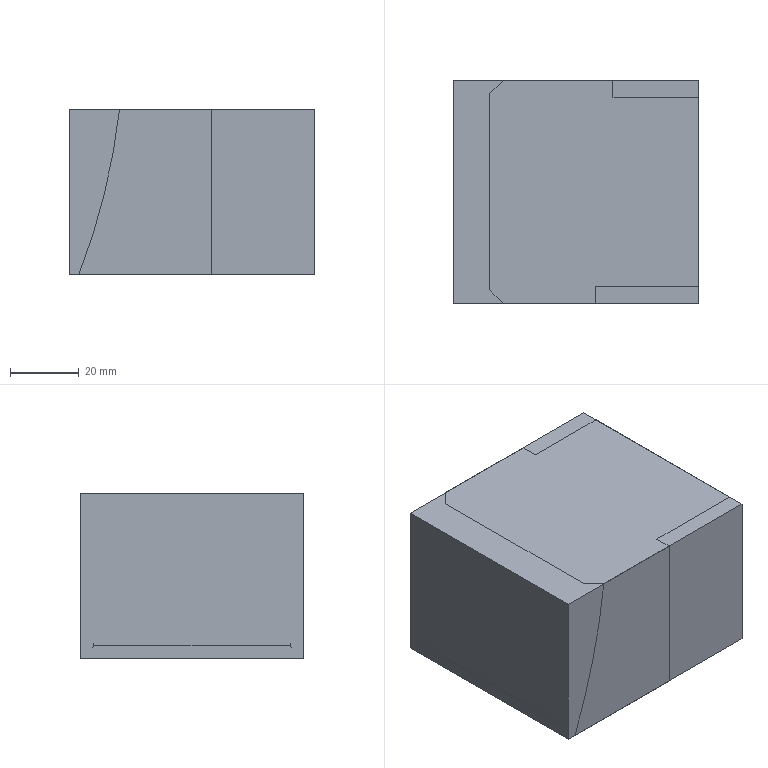NC program | NX | posted with a generic post | part box 71.51 x 65 x 48 mm
Lines 21 to 852 of 3379:
(ZLEVEL_PROFILE_COPY , TOOL : D10)
N40 T10 M6
N42 G54
N44 G17 G0 G90 X-28.587 Y-37.6 B0. C0. S9500 M3
N46 G43 Z30. H10
N48 Z1.5
N50 G94 G1 X-36.309 Z1.095 F2000.
N52 X-37.653 Y-37.266 Z1.023
N54 X-38.859 Y-36.584 Z0.95
N56 X-39.839 Y-35.604 Z0.877
N58 X-40.521 Y-34.398 Z0.805
N60 X-40.855 Y-33.054 Z0.732
N62 Y-32.5 Z0.703
N64 Y0. Z-1.
N66 Y32.5
N68 G2 X-35.755 Y37.6 R5.1
N70 G1 X35.755
N72 G2 X40.855 Y32.5 R5.1
N74 G1 Y-32.5
N76 G2 X35.755 Y-37.6 R5.1
N78 G1 X-35.755
N80 G2 X-40.855 Y-32.5 R5.1
N82 G1 Y0.
N84 Y32.5 Z-1.107
N86 X-40.83 Y33. Z-1.108
N88 X-40.757 Y33.495 Z-1.11
N90 X-40.635 Y33.98 Z-1.111
N92 X-40.467 Y34.452 Z-1.113
N94 X-40.253 Y34.904 Z-1.115
N96 X-39.996 Y35.333 Z-1.116
N98 X-39.697 Y35.735 Z-1.118
N100 X-39.361 Y36.106 Z-1.12
N102 X-38.99 Y36.442 Z-1.121
N104 X-38.588 Y36.74 Z-1.123
N106 X-38.159 Y36.998 Z-1.125
N108 X-37.707 Y37.212 Z-1.126
N110 X-37.235 Y37.38 Z-1.128
N112 X-36.75 Y37.502 Z-1.129
N114 X-36.255 Y37.575 Z-1.131
N116 X-35.755 Y37.6 Z-1.133
N118 X35.755 Z-1.367
N120 X36.255 Y37.575 Z-1.369
N122 X36.75 Y37.502 Z-1.371
N124 X37.235 Y37.38 Z-1.372
N126 X37.707 Y37.212 Z-1.374
N128 X38.159 Y36.998 Z-1.375
N130 X38.588 Y36.74 Z-1.377
N132 X38.99 Y36.442 Z-1.379
N134 X39.361 Y36.106 Z-1.38
N136 X39.697 Y35.735 Z-1.382
N138 X39.996 Y35.333 Z-1.384
N140 X40.253 Y34.904 Z-1.385
N142 X40.467 Y34.452 Z-1.387
N144 X40.635 Y33.98 Z-1.389
N146 X40.757 Y33.495 Z-1.39
N148 X40.83 Y33. Z-1.392
N150 X40.855 Y32.5 Z-1.393
N152 Y-32.5 Z-1.607
N154 X40.83 Y-33. Z-1.608
N156 X40.757 Y-33.495 Z-1.61
N158 X40.635 Y-33.98 Z-1.611
N160 X40.467 Y-34.452 Z-1.613
N162 X40.253 Y-34.904 Z-1.615
N164 X39.996 Y-35.333 Z-1.616
N166 X39.697 Y-35.735 Z-1.618
N168 X39.361 Y-36.106 Z-1.62
N170 X38.99 Y-36.442 Z-1.621
N172 X38.588 Y-36.74 Z-1.623
N174 X38.159 Y-36.998 Z-1.625
N176 X37.707 Y-37.212 Z-1.626
N178 X37.235 Y-37.38 Z-1.628
N180 X36.75 Y-37.502 Z-1.629
N182 X36.255 Y-37.575 Z-1.631
N184 X35.755 Y-37.6 Z-1.633
N186 X-35.755 Z-1.867
N188 X-36.255 Y-37.575 Z-1.869
N190 X-36.75 Y-37.502 Z-1.871
N192 X-37.235 Y-37.38 Z-1.872
N194 X-37.707 Y-37.212 Z-1.874
N196 X-38.159 Y-36.998 Z-1.875
N198 X-38.588 Y-36.74 Z-1.877
N200 X-38.99 Y-36.442 Z-1.879
N202 X-39.361 Y-36.106 Z-1.88
N204 X-39.697 Y-35.735 Z-1.882
N206 X-39.996 Y-35.333 Z-1.884
N208 X-40.253 Y-34.904 Z-1.885
N210 X-40.467 Y-34.452 Z-1.887
N212 X-40.635 Y-33.98 Z-1.889
N214 X-40.757 Y-33.495 Z-1.89
N216 X-40.83 Y-33. Z-1.892
N218 X-40.855 Y-32.5 Z-1.893
N220 Y0. Z-2.
N222 Y32.5 Z-2.107
N224 X-40.83 Y33. Z-2.108
N226 X-40.757 Y33.495 Z-2.11
N228 X-40.635 Y33.98 Z-2.111
N230 X-40.467 Y34.452 Z-2.113
N232 X-40.253 Y34.904 Z-2.115
N234 X-39.996 Y35.333 Z-2.116
N236 X-39.697 Y35.735 Z-2.118
N238 X-39.361 Y36.106 Z-2.12
N240 X-38.99 Y36.442 Z-2.121
N242 X-38.588 Y36.74 Z-2.123
N244 X-38.159 Y36.998 Z-2.125
N246 X-37.707 Y37.212 Z-2.126
N248 X-37.235 Y37.38 Z-2.128
N250 X-36.75 Y37.502 Z-2.129
N252 X-36.255 Y37.575 Z-2.131
N254 X-35.755 Y37.6 Z-2.133
N256 X35.755 Z-2.367
N258 X36.255 Y37.575 Z-2.369
N260 X36.75 Y37.502 Z-2.371
N262 X37.235 Y37.38 Z-2.372
N264 X37.707 Y37.212 Z-2.374
N266 X38.159 Y36.998 Z-2.375
N268 X38.588 Y36.74 Z-2.377
N270 X38.99 Y36.442 Z-2.379
N272 X39.361 Y36.106 Z-2.38
N274 X39.697 Y35.735 Z-2.382
N276 X39.996 Y35.333 Z-2.384
N278 X40.253 Y34.904 Z-2.385
N280 X40.467 Y34.452 Z-2.387
N282 X40.635 Y33.98 Z-2.389
N284 X40.757 Y33.495 Z-2.39
N286 X40.83 Y33. Z-2.392
N288 X40.855 Y32.5 Z-2.393
N290 Y-32.5 Z-2.607
N292 X40.83 Y-33. Z-2.608
N294 X40.757 Y-33.495 Z-2.61
N296 X40.635 Y-33.98 Z-2.611
N298 X40.467 Y-34.452 Z-2.613
N300 X40.253 Y-34.904 Z-2.615
N302 X39.996 Y-35.333 Z-2.616
N304 X39.697 Y-35.735 Z-2.618
N306 X39.361 Y-36.106 Z-2.62
N308 X38.99 Y-36.442 Z-2.621
N310 X38.588 Y-36.74 Z-2.623
N312 X38.159 Y-36.998 Z-2.625
N314 X37.707 Y-37.212 Z-2.626
N316 X37.235 Y-37.38 Z-2.628
N318 X36.75 Y-37.502 Z-2.629
N320 X36.255 Y-37.575 Z-2.631
N322 X35.755 Y-37.6 Z-2.633
N324 X-35.755 Z-2.867
N326 X-36.255 Y-37.575 Z-2.869
N328 X-36.75 Y-37.502 Z-2.871
N330 X-37.235 Y-37.38 Z-2.872
N332 X-37.707 Y-37.212 Z-2.874
N334 X-38.159 Y-36.998 Z-2.875
N336 X-38.588 Y-36.74 Z-2.877
N338 X-38.99 Y-36.442 Z-2.879
N340 X-39.361 Y-36.106 Z-2.88
N342 X-39.697 Y-35.735 Z-2.882
N344 X-39.996 Y-35.333 Z-2.884
N346 X-40.253 Y-34.904 Z-2.885
N348 X-40.467 Y-34.452 Z-2.887
N350 X-40.635 Y-33.98 Z-2.889
N352 X-40.757 Y-33.495 Z-2.89
N354 X-40.83 Y-33. Z-2.892
N356 X-40.855 Y-32.5 Z-2.893
N358 Y0. Z-3.
N360 Y32.5 Z-3.107
N362 X-40.83 Y33. Z-3.108
N364 X-40.757 Y33.495 Z-3.11
N366 X-40.635 Y33.98 Z-3.111
N368 X-40.467 Y34.452 Z-3.113
N370 X-40.253 Y34.904 Z-3.115
N372 X-39.996 Y35.333 Z-3.116
N374 X-39.697 Y35.735 Z-3.118
N376 X-39.361 Y36.106 Z-3.12
N378 X-38.99 Y36.442 Z-3.121
N380 X-38.588 Y36.74 Z-3.123
N382 X-38.159 Y36.998 Z-3.125
N384 X-37.707 Y37.212 Z-3.126
N386 X-37.235 Y37.38 Z-3.128
N388 X-36.75 Y37.502 Z-3.129
N390 X-36.255 Y37.575 Z-3.131
N392 X-35.755 Y37.6 Z-3.133
N394 X35.755 Z-3.367
N396 X36.255 Y37.575 Z-3.369
N398 X36.75 Y37.502 Z-3.371
N400 X37.235 Y37.38 Z-3.372
N402 X37.707 Y37.212 Z-3.374
N404 X38.159 Y36.998 Z-3.375
N406 X38.588 Y36.74 Z-3.377
N408 X38.99 Y36.442 Z-3.379
N410 X39.361 Y36.106 Z-3.38
N412 X39.697 Y35.735 Z-3.382
N414 X39.996 Y35.333 Z-3.384
N416 X40.253 Y34.904 Z-3.385
N418 X40.467 Y34.452 Z-3.387
N420 X40.635 Y33.98 Z-3.389
N422 X40.757 Y33.495 Z-3.39
N424 X40.83 Y33. Z-3.392
N426 X40.855 Y32.5 Z-3.393
N428 Y-32.5 Z-3.607
N430 X40.83 Y-33. Z-3.608
N432 X40.757 Y-33.495 Z-3.61
N434 X40.635 Y-33.98 Z-3.611
N436 X40.467 Y-34.452 Z-3.613
N438 X40.253 Y-34.904 Z-3.615
N440 X39.996 Y-35.333 Z-3.616
N442 X39.697 Y-35.735 Z-3.618
N444 X39.361 Y-36.106 Z-3.62
N446 X38.99 Y-36.442 Z-3.621
N448 X38.588 Y-36.74 Z-3.623
N450 X38.159 Y-36.998 Z-3.625
N452 X37.707 Y-37.212 Z-3.626
N454 X37.235 Y-37.38 Z-3.628
N456 X36.75 Y-37.502 Z-3.629
N458 X36.255 Y-37.575 Z-3.631
N460 X35.755 Y-37.6 Z-3.633
N462 X-35.755 Z-3.867
N464 X-36.255 Y-37.575 Z-3.869
N466 X-36.75 Y-37.502 Z-3.871
N468 X-37.235 Y-37.38 Z-3.872
N470 X-37.707 Y-37.212 Z-3.874
N472 X-38.159 Y-36.998 Z-3.875
N474 X-38.588 Y-36.74 Z-3.877
N476 X-38.99 Y-36.442 Z-3.879
N478 X-39.361 Y-36.106 Z-3.88
N480 X-39.697 Y-35.735 Z-3.882
N482 X-39.996 Y-35.333 Z-3.884
N484 X-40.253 Y-34.904 Z-3.885
N486 X-40.467 Y-34.452 Z-3.887
N488 X-40.635 Y-33.98 Z-3.889
N490 X-40.757 Y-33.495 Z-3.89
N492 X-40.83 Y-33. Z-3.892
N494 X-40.855 Y-32.5 Z-3.893
N496 Y0. Z-4.
N498 Y32.5 Z-4.107
N500 X-40.83 Y33. Z-4.108
N502 X-40.757 Y33.495 Z-4.11
N504 X-40.635 Y33.98 Z-4.111
N506 X-40.467 Y34.452 Z-4.113
N508 X-40.253 Y34.904 Z-4.115
N510 X-39.996 Y35.333 Z-4.116
N512 X-39.697 Y35.735 Z-4.118
N514 X-39.361 Y36.106 Z-4.12
N516 X-38.99 Y36.442 Z-4.121
N518 X-38.588 Y36.74 Z-4.123
N520 X-38.159 Y36.998 Z-4.125
N522 X-37.707 Y37.212 Z-4.126
N524 X-37.235 Y37.38 Z-4.128
N526 X-36.75 Y37.502 Z-4.129
N528 X-36.255 Y37.575 Z-4.131
N530 X-35.755 Y37.6 Z-4.133
N532 X35.755 Z-4.367
N534 X36.255 Y37.575 Z-4.369
N536 X36.75 Y37.502 Z-4.371
N538 X37.235 Y37.38 Z-4.372
N540 X37.707 Y37.212 Z-4.374
N542 X38.159 Y36.998 Z-4.375
N544 X38.588 Y36.74 Z-4.377
N546 X38.99 Y36.442 Z-4.379
N548 X39.361 Y36.106 Z-4.38
N550 X39.697 Y35.735 Z-4.382
N552 X39.996 Y35.333 Z-4.384
N554 X40.253 Y34.904 Z-4.385
N556 X40.467 Y34.452 Z-4.387
N558 X40.635 Y33.98 Z-4.389
N560 X40.757 Y33.495 Z-4.39
N562 X40.83 Y33. Z-4.392
N564 X40.855 Y32.5 Z-4.393
N566 Y-32.5 Z-4.607
N568 X40.83 Y-33. Z-4.608
N570 X40.757 Y-33.495 Z-4.61
N572 X40.635 Y-33.98 Z-4.611
N574 X40.467 Y-34.452 Z-4.613
N576 X40.253 Y-34.904 Z-4.615
N578 X39.996 Y-35.333 Z-4.616
N580 X39.697 Y-35.735 Z-4.618
N582 X39.361 Y-36.106 Z-4.62
N584 X38.99 Y-36.442 Z-4.621
N586 X38.588 Y-36.74 Z-4.623
N588 X38.159 Y-36.998 Z-4.625
N590 X37.707 Y-37.212 Z-4.626
N592 X37.235 Y-37.38 Z-4.628
N594 X36.75 Y-37.502 Z-4.629
N596 X36.255 Y-37.575 Z-4.631
N598 X35.755 Y-37.6 Z-4.633
N600 X-35.755 Z-4.867
N602 X-36.255 Y-37.575 Z-4.869
N604 X-36.75 Y-37.502 Z-4.871
N606 X-37.235 Y-37.38 Z-4.872
N608 X-37.707 Y-37.212 Z-4.874
N610 X-38.159 Y-36.998 Z-4.875
N612 X-38.588 Y-36.74 Z-4.877
N614 X-38.99 Y-36.442 Z-4.879
N616 X-39.361 Y-36.106 Z-4.88
N618 X-39.697 Y-35.735 Z-4.882
N620 X-39.996 Y-35.333 Z-4.884
N622 X-40.253 Y-34.904 Z-4.885
N624 X-40.467 Y-34.452 Z-4.887
N626 X-40.635 Y-33.98 Z-4.889
N628 X-40.757 Y-33.495 Z-4.89
N630 X-40.83 Y-33. Z-4.892
N632 X-40.855 Y-32.5 Z-4.893
N634 Y0. Z-5.
N636 Y32.5 Z-5.107
N638 X-40.83 Y33. Z-5.108
N640 X-40.757 Y33.495 Z-5.11
N642 X-40.635 Y33.98 Z-5.111
N644 X-40.467 Y34.452 Z-5.113
N646 X-40.253 Y34.904 Z-5.115
N648 X-39.996 Y35.333 Z-5.116
N650 X-39.697 Y35.735 Z-5.118
N652 X-39.361 Y36.106 Z-5.12
N654 X-38.99 Y36.442 Z-5.121
N656 X-38.588 Y36.74 Z-5.123
N658 X-38.159 Y36.998 Z-5.125
N660 X-37.707 Y37.212 Z-5.126
N662 X-37.235 Y37.38 Z-5.128
N664 X-36.75 Y37.502 Z-5.129
N666 X-36.255 Y37.575 Z-5.131
N668 X-35.755 Y37.6 Z-5.133
N670 X35.755 Z-5.367
N672 X36.255 Y37.575 Z-5.369
N674 X36.75 Y37.502 Z-5.371
N676 X37.235 Y37.38 Z-5.372
N678 X37.707 Y37.212 Z-5.374
N680 X38.159 Y36.998 Z-5.375
N682 X38.588 Y36.74 Z-5.377
N684 X38.99 Y36.442 Z-5.379
N686 X39.361 Y36.106 Z-5.38
N688 X39.697 Y35.735 Z-5.382
N690 X39.996 Y35.333 Z-5.384
N692 X40.253 Y34.904 Z-5.385
N694 X40.467 Y34.452 Z-5.387
N696 X40.635 Y33.98 Z-5.389
N698 X40.757 Y33.495 Z-5.39
N700 X40.83 Y33. Z-5.392
N702 X40.855 Y32.5 Z-5.393
N704 Y-32.5 Z-5.607
N706 X40.83 Y-33. Z-5.608
N708 X40.757 Y-33.495 Z-5.61
N710 X40.635 Y-33.98 Z-5.611
N712 X40.467 Y-34.452 Z-5.613
N714 X40.253 Y-34.904 Z-5.615
N716 X39.996 Y-35.333 Z-5.616
N718 X39.697 Y-35.735 Z-5.618
N720 X39.361 Y-36.106 Z-5.62
N722 X38.99 Y-36.442 Z-5.621
N724 X38.588 Y-36.74 Z-5.623
N726 X38.159 Y-36.998 Z-5.625
N728 X37.707 Y-37.212 Z-5.626
N730 X37.235 Y-37.38 Z-5.628
N732 X36.75 Y-37.502 Z-5.629
N734 X36.255 Y-37.575 Z-5.631
N736 X35.755 Y-37.6 Z-5.633
N738 X-35.755 Z-5.867
N740 X-36.255 Y-37.575 Z-5.869
N742 X-36.75 Y-37.502 Z-5.871
N744 X-37.235 Y-37.38 Z-5.872
N746 X-37.707 Y-37.212 Z-5.874
N748 X-38.159 Y-36.998 Z-5.875
N750 X-38.588 Y-36.74 Z-5.877
N752 X-38.99 Y-36.442 Z-5.879
N754 X-39.361 Y-36.106 Z-5.88
N756 X-39.697 Y-35.735 Z-5.882
N758 X-39.996 Y-35.333 Z-5.884
N760 X-40.253 Y-34.904 Z-5.885
N762 X-40.467 Y-34.452 Z-5.887
N764 X-40.635 Y-33.98 Z-5.889
N766 X-40.757 Y-33.495 Z-5.89
N768 X-40.83 Y-33. Z-5.892
N770 X-40.855 Y-32.5 Z-5.893
N772 Y0. Z-6.
N774 Y32.5 Z-6.107
N776 X-40.83 Y33. Z-6.108
N778 X-40.757 Y33.495 Z-6.11
N780 X-40.635 Y33.98 Z-6.111
N782 X-40.467 Y34.452 Z-6.113
N784 X-40.253 Y34.904 Z-6.115
N786 X-39.996 Y35.333 Z-6.116
N788 X-39.697 Y35.735 Z-6.118
N790 X-39.361 Y36.106 Z-6.12
N792 X-38.99 Y36.442 Z-6.121
N794 X-38.588 Y36.74 Z-6.123
N796 X-38.159 Y36.998 Z-6.125
N798 X-37.707 Y37.212 Z-6.126
N800 X-37.235 Y37.38 Z-6.128
N802 X-36.75 Y37.502 Z-6.129
N804 X-36.255 Y37.575 Z-6.131
N806 X-35.755 Y37.6 Z-6.133
N808 X35.755 Z-6.367
N810 X36.255 Y37.575 Z-6.369
N812 X36.75 Y37.502 Z-6.371
N814 X37.235 Y37.38 Z-6.372
N816 X37.707 Y37.212 Z-6.374
N818 X38.159 Y36.998 Z-6.375
N820 X38.588 Y36.74 Z-6.377
N822 X38.99 Y36.442 Z-6.379
N824 X39.361 Y36.106 Z-6.38
N826 X39.697 Y35.735 Z-6.382
N828 X39.996 Y35.333 Z-6.384
N830 X40.253 Y34.904 Z-6.385
N832 X40.467 Y34.452 Z-6.387
N834 X40.635 Y33.98 Z-6.389
N836 X40.757 Y33.495 Z-6.39
N838 X40.83 Y33. Z-6.392
N840 X40.855 Y32.5 Z-6.393
N842 Y-32.5 Z-6.607
N844 X40.83 Y-33. Z-6.608
N846 X40.757 Y-33.495 Z-6.61
N848 X40.635 Y-33.98 Z-6.611
N850 X40.467 Y-34.452 Z-6.613
N852 X40.253 Y-34.904 Z-6.615
N854 X39.996 Y-35.333 Z-6.616
N856 X39.697 Y-35.735 Z-6.618
N858 X39.361 Y-36.106 Z-6.62
N860 X38.99 Y-36.442 Z-6.621
N862 X38.588 Y-36.74 Z-6.623
N864 X38.159 Y-36.998 Z-6.625
N866 X37.707 Y-37.212 Z-6.626
N868 X37.235 Y-37.38 Z-6.628
N870 X36.75 Y-37.502 Z-6.629
N872 X36.255 Y-37.575 Z-6.631
N874 X35.755 Y-37.6 Z-6.633
N876 X-35.755 Z-6.867
N878 X-36.255 Y-37.575 Z-6.869
N880 X-36.75 Y-37.502 Z-6.871
N882 X-37.235 Y-37.38 Z-6.872
N884 X-37.707 Y-37.212 Z-6.874
N886 X-38.159 Y-36.998 Z-6.875
N888 X-38.588 Y-36.74 Z-6.877
N890 X-38.99 Y-36.442 Z-6.879
N892 X-39.361 Y-36.106 Z-6.88
N894 X-39.697 Y-35.735 Z-6.882
N896 X-39.996 Y-35.333 Z-6.884
N898 X-40.253 Y-34.904 Z-6.885
N900 X-40.467 Y-34.452 Z-6.887
N902 X-40.635 Y-33.98 Z-6.889
N904 X-40.757 Y-33.495 Z-6.89
N906 X-40.83 Y-33. Z-6.892
N908 X-40.855 Y-32.5 Z-6.893
N910 Y0. Z-7.
N912 Y32.5 Z-7.107
N914 X-40.83 Y33. Z-7.108
N916 X-40.757 Y33.495 Z-7.11
N918 X-40.635 Y33.98 Z-7.111
N920 X-40.467 Y34.452 Z-7.113
N922 X-40.253 Y34.904 Z-7.115
N924 X-39.996 Y35.333 Z-7.116
N926 X-39.697 Y35.735 Z-7.118
N928 X-39.361 Y36.106 Z-7.12
N930 X-38.99 Y36.442 Z-7.121
N932 X-38.588 Y36.74 Z-7.123
N934 X-38.159 Y36.998 Z-7.125
N936 X-37.707 Y37.212 Z-7.126
N938 X-37.235 Y37.38 Z-7.128
N940 X-36.75 Y37.502 Z-7.129
N942 X-36.255 Y37.575 Z-7.131
N944 X-35.755 Y37.6 Z-7.133
N946 X35.755 Z-7.367
N948 X36.255 Y37.575 Z-7.369
N950 X36.75 Y37.502 Z-7.371
N952 X37.235 Y37.38 Z-7.372
N954 X37.707 Y37.212 Z-7.374
N956 X38.159 Y36.998 Z-7.375
N958 X38.588 Y36.74 Z-7.377
N960 X38.99 Y36.442 Z-7.379
N962 X39.361 Y36.106 Z-7.38
N964 X39.697 Y35.735 Z-7.382
N966 X39.996 Y35.333 Z-7.384
N968 X40.253 Y34.904 Z-7.385
N970 X40.467 Y34.452 Z-7.387
N972 X40.635 Y33.98 Z-7.389
N974 X40.757 Y33.495 Z-7.39
N976 X40.83 Y33. Z-7.392
N978 X40.855 Y32.5 Z-7.393
N980 Y-32.5 Z-7.607
N982 X40.83 Y-33. Z-7.608
N984 X40.757 Y-33.495 Z-7.61
N986 X40.635 Y-33.98 Z-7.611
N988 X40.467 Y-34.452 Z-7.613
N990 X40.253 Y-34.904 Z-7.615
N992 X39.996 Y-35.333 Z-7.616
N994 X39.697 Y-35.735 Z-7.618
N996 X39.361 Y-36.106 Z-7.62
N998 X38.99 Y-36.442 Z-7.621
N1000 X38.588 Y-36.74 Z-7.623
N1002 X38.159 Y-36.998 Z-7.625
N1004 X37.707 Y-37.212 Z-7.626
N1006 X37.235 Y-37.38 Z-7.628
N1008 X36.75 Y-37.502 Z-7.629
N1010 X36.255 Y-37.575 Z-7.631
N1012 X35.755 Y-37.6 Z-7.633
N1014 X-35.755 Z-7.867
N1016 X-36.255 Y-37.575 Z-7.869
N1018 X-36.75 Y-37.502 Z-7.871
N1020 X-37.235 Y-37.38 Z-7.872
N1022 X-37.707 Y-37.212 Z-7.874
N1024 X-38.159 Y-36.998 Z-7.875
N1026 X-38.588 Y-36.74 Z-7.877
N1028 X-38.99 Y-36.442 Z-7.879
N1030 X-39.361 Y-36.106 Z-7.88
N1032 X-39.697 Y-35.735 Z-7.882
N1034 X-39.996 Y-35.333 Z-7.884
N1036 X-40.253 Y-34.904 Z-7.885
N1038 X-40.467 Y-34.452 Z-7.887
N1040 X-40.635 Y-33.98 Z-7.889
N1042 X-40.757 Y-33.495 Z-7.89
N1044 X-40.83 Y-33. Z-7.892
N1046 X-40.855 Y-32.5 Z-7.893
N1048 Y0. Z-8.
N1050 Y32.5 Z-8.107
N1052 X-40.83 Y33. Z-8.108
N1054 X-40.757 Y33.495 Z-8.11
N1056 X-40.635 Y33.98 Z-8.111
N1058 X-40.467 Y34.452 Z-8.113
N1060 X-40.253 Y34.904 Z-8.115
N1062 X-39.996 Y35.333 Z-8.116
N1064 X-39.697 Y35.735 Z-8.118
N1066 X-39.361 Y36.106 Z-8.12
N1068 X-38.99 Y36.442 Z-8.121
N1070 X-38.588 Y36.74 Z-8.123
N1072 X-38.159 Y36.998 Z-8.125
N1074 X-37.707 Y37.212 Z-8.126
N1076 X-37.235 Y37.38 Z-8.128
N1078 X-36.75 Y37.502 Z-8.129
N1080 X-36.255 Y37.575 Z-8.131
N1082 X-35.755 Y37.6 Z-8.133
N1084 X35.755 Z-8.367
N1086 X36.255 Y37.575 Z-8.369
N1088 X36.75 Y37.502 Z-8.371
N1090 X37.235 Y37.38 Z-8.372
N1092 X37.707 Y37.212 Z-8.374
N1094 X38.159 Y36.998 Z-8.375
N1096 X38.588 Y36.74 Z-8.377
N1098 X38.99 Y36.442 Z-8.379
N1100 X39.361 Y36.106 Z-8.38
N1102 X39.697 Y35.735 Z-8.382
N1104 X39.996 Y35.333 Z-8.384
N1106 X40.253 Y34.904 Z-8.385
N1108 X40.467 Y34.452 Z-8.387
N1110 X40.635 Y33.98 Z-8.389
N1112 X40.757 Y33.495 Z-8.39
N1114 X40.83 Y33. Z-8.392
N1116 X40.855 Y32.5 Z-8.393
N1118 Y-32.5 Z-8.607
N1120 X40.83 Y-33. Z-8.608
N1122 X40.757 Y-33.495 Z-8.61
N1124 X40.635 Y-33.98 Z-8.611
N1126 X40.467 Y-34.452 Z-8.613
N1128 X40.253 Y-34.904 Z-8.615
N1130 X39.996 Y-35.333 Z-8.616
N1132 X39.697 Y-35.735 Z-8.618
N1134 X39.361 Y-36.106 Z-8.62
N1136 X38.99 Y-36.442 Z-8.621
N1138 X38.588 Y-36.74 Z-8.623
N1140 X38.159 Y-36.998 Z-8.625
N1142 X37.707 Y-37.212 Z-8.626
N1144 X37.235 Y-37.38 Z-8.628
N1146 X36.75 Y-37.502 Z-8.629
N1148 X36.255 Y-37.575 Z-8.631
N1150 X35.755 Y-37.6 Z-8.633
N1152 X-35.755 Z-8.867
N1154 X-36.255 Y-37.575 Z-8.869
N1156 X-36.75 Y-37.502 Z-8.871
N1158 X-37.235 Y-37.38 Z-8.872
N1160 X-37.707 Y-37.212 Z-8.874
N1162 X-38.159 Y-36.998 Z-8.875
N1164 X-38.588 Y-36.74 Z-8.877
N1166 X-38.99 Y-36.442 Z-8.879
N1168 X-39.361 Y-36.106 Z-8.88
N1170 X-39.697 Y-35.735 Z-8.882
N1172 X-39.996 Y-35.333 Z-8.884
N1174 X-40.253 Y-34.904 Z-8.885
N1176 X-40.467 Y-34.452 Z-8.887
N1178 X-40.635 Y-33.98 Z-8.889
N1180 X-40.757 Y-33.495 Z-8.89
N1182 X-40.83 Y-33. Z-8.892
N1184 X-40.855 Y-32.5 Z-8.893
N1186 Y0. Z-9.
N1188 Y32.5 Z-9.107
N1190 X-40.83 Y33. Z-9.108
N1192 X-40.757 Y33.495 Z-9.11
N1194 X-40.635 Y33.98 Z-9.111
N1196 X-40.467 Y34.452 Z-9.113
N1198 X-40.253 Y34.904 Z-9.115
N1200 X-39.996 Y35.333 Z-9.116
N1202 X-39.697 Y35.735 Z-9.118
N1204 X-39.361 Y36.106 Z-9.12
N1206 X-38.99 Y36.442 Z-9.121
N1208 X-38.588 Y36.74 Z-9.123
N1210 X-38.159 Y36.998 Z-9.125
N1212 X-37.707 Y37.212 Z-9.126
N1214 X-37.235 Y37.38 Z-9.128
N1216 X-36.75 Y37.502 Z-9.129
N1218 X-36.255 Y37.575 Z-9.131
N1220 X-35.755 Y37.6 Z-9.133
N1222 X35.755 Z-9.367
N1224 X36.255 Y37.575 Z-9.369
N1226 X36.75 Y37.502 Z-9.371
N1228 X37.235 Y37.38 Z-9.372
N1230 X37.707 Y37.212 Z-9.374
N1232 X38.159 Y36.998 Z-9.375
N1234 X38.588 Y36.74 Z-9.377
N1236 X38.99 Y36.442 Z-9.379
N1238 X39.361 Y36.106 Z-9.38
N1240 X39.697 Y35.735 Z-9.382
N1242 X39.996 Y35.333 Z-9.384
N1244 X40.253 Y34.904 Z-9.385
N1246 X40.467 Y34.452 Z-9.387
N1248 X40.635 Y33.98 Z-9.389
N1250 X40.757 Y33.495 Z-9.39
N1252 X40.83 Y33. Z-9.392
N1254 X40.855 Y32.5 Z-9.393
N1256 Y-32.5 Z-9.607
N1258 X40.83 Y-33. Z-9.608
N1260 X40.757 Y-33.495 Z-9.61
N1262 X40.635 Y-33.98 Z-9.611
N1264 X40.467 Y-34.452 Z-9.613
N1266 X40.253 Y-34.904 Z-9.615
N1268 X39.996 Y-35.333 Z-9.616
N1270 X39.697 Y-35.735 Z-9.618
N1272 X39.361 Y-36.106 Z-9.62
N1274 X38.99 Y-36.442 Z-9.621
N1276 X38.588 Y-36.74 Z-9.623
N1278 X38.159 Y-36.998 Z-9.625
N1280 X37.707 Y-37.212 Z-9.626
N1282 X37.235 Y-37.38 Z-9.628
N1284 X36.75 Y-37.502 Z-9.629
N1286 X36.255 Y-37.575 Z-9.631
N1288 X35.755 Y-37.6 Z-9.633
N1290 X-35.755 Z-9.867
N1292 X-36.255 Y-37.575 Z-9.869
N1294 X-36.75 Y-37.502 Z-9.871
N1296 X-37.235 Y-37.38 Z-9.872
N1298 X-37.707 Y-37.212 Z-9.874
N1300 X-38.159 Y-36.998 Z-9.875
N1302 X-38.588 Y-36.74 Z-9.877
N1304 X-38.99 Y-36.442 Z-9.879
N1306 X-39.361 Y-36.106 Z-9.88
N1308 X-39.697 Y-35.735 Z-9.882
N1310 X-39.996 Y-35.333 Z-9.884
N1312 X-40.253 Y-34.904 Z-9.885
N1314 X-40.467 Y-34.452 Z-9.887
N1316 X-40.635 Y-33.98 Z-9.889
N1318 X-40.757 Y-33.495 Z-9.89
N1320 X-40.83 Y-33. Z-9.892
N1322 X-40.855 Y-32.5 Z-9.893
N1324 Y0. Z-10.
N1326 Y32.5 Z-10.107
N1328 X-40.83 Y33. Z-10.108
N1330 X-40.757 Y33.495 Z-10.11
N1332 X-40.635 Y33.98 Z-10.111
N1334 X-40.467 Y34.452 Z-10.113
N1336 X-40.253 Y34.904 Z-10.115
N1338 X-39.996 Y35.333 Z-10.116
N1340 X-39.697 Y35.735 Z-10.118
N1342 X-39.361 Y36.106 Z-10.12
N1344 X-38.99 Y36.442 Z-10.121
N1346 X-38.588 Y36.74 Z-10.123
N1348 X-38.159 Y36.998 Z-10.125
N1350 X-37.707 Y37.212 Z-10.126
N1352 X-37.235 Y37.38 Z-10.128
N1354 X-36.75 Y37.502 Z-10.129
N1356 X-36.255 Y37.575 Z-10.131
N1358 X-35.755 Y37.6 Z-10.133
N1360 X35.755 Z-10.367
N1362 X36.255 Y37.575 Z-10.369
N1364 X36.75 Y37.502 Z-10.371
N1366 X37.235 Y37.38 Z-10.372
N1368 X37.707 Y37.212 Z-10.374
N1370 X38.159 Y36.998 Z-10.375
N1372 X38.588 Y36.74 Z-10.377
N1374 X38.99 Y36.442 Z-10.379
N1376 X39.361 Y36.106 Z-10.38
N1378 X39.697 Y35.735 Z-10.382
N1380 X39.996 Y35.333 Z-10.384
N1382 X40.253 Y34.904 Z-10.385
N1384 X40.467 Y34.452 Z-10.387
N1386 X40.635 Y33.98 Z-10.389
N1388 X40.757 Y33.495 Z-10.39
N1390 X40.83 Y33. Z-10.392
N1392 X40.855 Y32.5 Z-10.393
N1394 Y-32.5 Z-10.607
N1396 X40.83 Y-33. Z-10.608
N1398 X40.757 Y-33.495 Z-10.61
N1400 X40.635 Y-33.98 Z-10.611
N1402 X40.467 Y-34.452 Z-10.613
N1404 X40.253 Y-34.904 Z-10.615
N1406 X39.996 Y-35.333 Z-10.616
N1408 X39.697 Y-35.735 Z-10.618
N1410 X39.361 Y-36.106 Z-10.62
N1412 X38.99 Y-36.442 Z-10.621
N1414 X38.588 Y-36.74 Z-10.623
N1416 X38.159 Y-36.998 Z-10.625
N1418 X37.707 Y-37.212 Z-10.626
N1420 X37.235 Y-37.38 Z-10.628
N1422 X36.75 Y-37.502 Z-10.629
N1424 X36.255 Y-37.575 Z-10.631
N1426 X35.755 Y-37.6 Z-10.633
N1428 X-35.755 Z-10.867
N1430 X-36.255 Y-37.575 Z-10.869
N1432 X-36.75 Y-37.502 Z-10.87
N1434 X-37.235 Y-37.38 Z-10.872
N1436 X-37.707 Y-37.212 Z-10.874
N1438 X-38.159 Y-36.998 Z-10.875
N1440 X-38.588 Y-36.74 Z-10.877
N1442 X-38.99 Y-36.442 Z-10.879
N1444 X-39.361 Y-36.106 Z-10.88
N1446 X-39.697 Y-35.735 Z-10.882
N1448 X-39.996 Y-35.333 Z-10.884
N1450 X-40.253 Y-34.904 Z-10.885
N1452 X-40.467 Y-34.452 Z-10.887
N1454 X-40.635 Y-33.98 Z-10.889
N1456 X-40.757 Y-33.495 Z-10.89
N1458 X-40.83 Y-33. Z-10.892
N1460 X-40.855 Y-32.5 Z-10.893
N1462 Y0. Z-11.
N1464 Y32.5 Z-11.107
N1466 X-40.83 Y33. Z-11.108
N1468 X-40.757 Y33.495 Z-11.11
N1470 X-40.635 Y33.98 Z-11.111
N1472 X-40.467 Y34.452 Z-11.113
N1474 X-40.253 Y34.904 Z-11.115
N1476 X-39.996 Y35.333 Z-11.116
N1478 X-39.697 Y35.735 Z-11.118
N1480 X-39.361 Y36.106 Z-11.12
N1482 X-38.99 Y36.442 Z-11.121
N1484 X-38.588 Y36.74 Z-11.123
N1486 X-38.159 Y36.998 Z-11.125
N1488 X-37.707 Y37.212 Z-11.126
N1490 X-37.235 Y37.38 Z-11.128
N1492 X-36.75 Y37.502 Z-11.129
N1494 X-36.255 Y37.575 Z-11.131
N1496 X-35.755 Y37.6 Z-11.133
N1498 X35.755 Z-11.367
N1500 X36.255 Y37.575 Z-11.369
N1502 X36.75 Y37.502 Z-11.37
N1504 X37.235 Y37.38 Z-11.372
N1506 X37.707 Y37.212 Z-11.374
N1508 X38.159 Y36.998 Z-11.375
N1510 X38.588 Y36.74 Z-11.377
N1512 X38.99 Y36.442 Z-11.379
N1514 X39.361 Y36.106 Z-11.38
N1516 X39.697 Y35.735 Z-11.382
N1518 X39.996 Y35.333 Z-11.384
N1520 X40.253 Y34.904 Z-11.385
N1522 X40.467 Y34.452 Z-11.387
N1524 X40.635 Y33.98 Z-11.389
N1526 X40.757 Y33.495 Z-11.39
N1528 X40.83 Y33. Z-11.392
N1530 X40.855 Y32.5 Z-11.393
N1532 Y-32.5 Z-11.607
N1534 X40.83 Y-33. Z-11.608
N1536 X40.757 Y-33.495 Z-11.61
N1538 X40.635 Y-33.98 Z-11.611
N1540 X40.467 Y-34.452 Z-11.613
N1542 X40.253 Y-34.904 Z-11.615
N1544 X39.996 Y-35.333 Z-11.616
N1546 X39.697 Y-35.735 Z-11.618
N1548 X39.361 Y-36.106 Z-11.62
N1550 X38.99 Y-36.442 Z-11.621
N1552 X38.588 Y-36.74 Z-11.623
N1554 X38.159 Y-36.998 Z-11.625
N1556 X37.707 Y-37.212 Z-11.626
N1558 X37.235 Y-37.38 Z-11.628
N1560 X36.75 Y-37.502 Z-11.629
N1562 X36.255 Y-37.575 Z-11.631
N1564 X35.755 Y-37.6 Z-11.633
N1566 X-35.755 Z-11.867
N1568 X-36.255 Y-37.575 Z-11.869
N1570 X-36.75 Y-37.502 Z-11.87
N1572 X-37.235 Y-37.38 Z-11.872
N1574 X-37.707 Y-37.212 Z-11.874
N1576 X-38.159 Y-36.998 Z-11.875
N1578 X-38.588 Y-36.74 Z-11.877
N1580 X-38.99 Y-36.442 Z-11.879
N1582 X-39.361 Y-36.106 Z-11.88
N1584 X-39.697 Y-35.735 Z-11.882
N1586 X-39.996 Y-35.333 Z-11.884
N1588 X-40.253 Y-34.904 Z-11.885
N1590 X-40.467 Y-34.452 Z-11.887
N1592 X-40.635 Y-33.98 Z-11.889
N1594 X-40.757 Y-33.495 Z-11.89
N1596 X-40.83 Y-33. Z-11.892
N1598 X-40.855 Y-32.5 Z-11.893
N1600 Y0. Z-12.
N1602 Y32.5 Z-12.107
N1604 X-40.83 Y33. Z-12.108
N1606 X-40.757 Y33.495 Z-12.11
N1608 X-40.635 Y33.98 Z-12.111
N1610 X-40.467 Y34.452 Z-12.113
N1612 X-40.253 Y34.904 Z-12.115
N1614 X-39.996 Y35.333 Z-12.116
N1616 X-39.697 Y35.735 Z-12.118
N1618 X-39.361 Y36.106 Z-12.12
N1620 X-38.99 Y36.442 Z-12.121
N1622 X-38.588 Y36.74 Z-12.123
N1624 X-38.159 Y36.998 Z-12.125
N1626 X-37.707 Y37.212 Z-12.126
N1628 X-37.235 Y37.38 Z-12.128
N1630 X-36.75 Y37.502 Z-12.129
N1632 X-36.255 Y37.575 Z-12.131
N1634 X-35.755 Y37.6 Z-12.133
N1636 X35.755 Z-12.367
N1638 X36.255 Y37.575 Z-12.369
N1640 X36.75 Y37.502 Z-12.37
N1642 X37.235 Y37.38 Z-12.372
N1644 X37.707 Y37.212 Z-12.374
N1646 X38.159 Y36.998 Z-12.375
N1648 X38.588 Y36.74 Z-12.377
N1650 X38.99 Y36.442 Z-12.379
N1652 X39.361 Y36.106 Z-12.38
N1654 X39.697 Y35.735 Z-12.382
N1656 X39.996 Y35.333 Z-12.384
N1658 X40.253 Y34.904 Z-12.385
N1660 X40.467 Y34.452 Z-12.387
N1662 X40.635 Y33.98 Z-12.389
N1664 X40.757 Y33.495 Z-12.39
N1666 X40.83 Y33. Z-12.392
N1668 X40.855 Y32.5 Z-12.393
N1670 Y-32.5 Z-12.607
N1672 X40.83 Y-33. Z-12.608
N1674 X40.757 Y-33.495 Z-12.61
N1676 X40.635 Y-33.98 Z-12.611
N1678 X40.467 Y-34.452 Z-12.613
N1680 X40.253 Y-34.904 Z-12.615
N1682 X39.996 Y-35.333 Z-12.616
N1684 X39.697 Y-35.735 Z-12.618
N1686 X39.361 Y-36.106 Z-12.62
N1688 X38.99 Y-36.442 Z-12.621
N1690 X38.588 Y-36.74 Z-12.623
N1692 X38.159 Y-36.998 Z-12.625
N1694 X37.707 Y-37.212 Z-12.626
N1696 X37.235 Y-37.38 Z-12.628